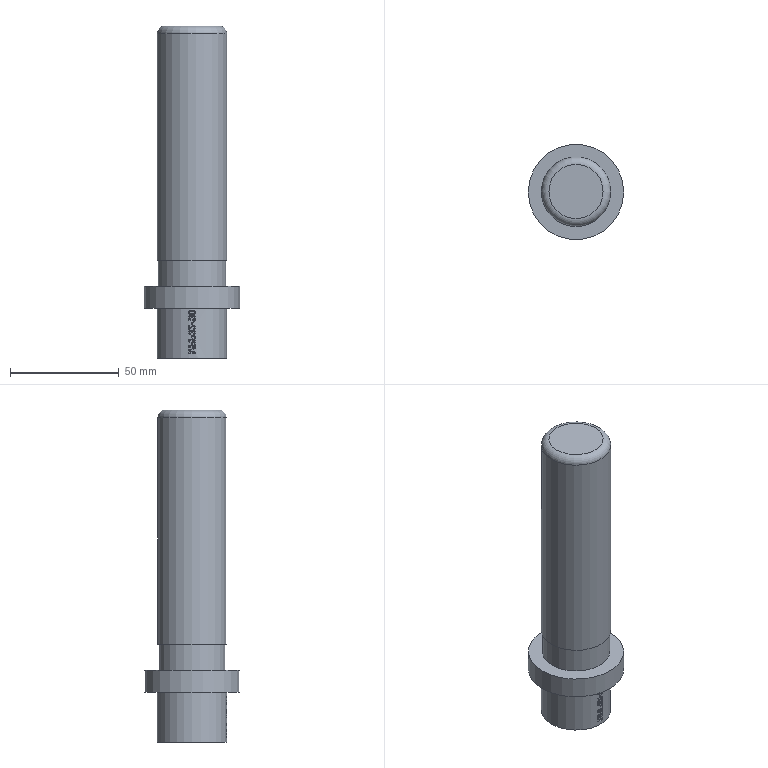Part | STEP file | PN_0057_id1194_x_t | 1 solid | 130 faces | box 44 x 44 x 153 mm | volume 127630 mm3 | plane 71 | cylinder 56 | cone 2 | torus 1 | commonest cylinder face diameters 31.8 x9 32 x5 1.809 x4 1.063 x2 1.246 x2 1.365 x2